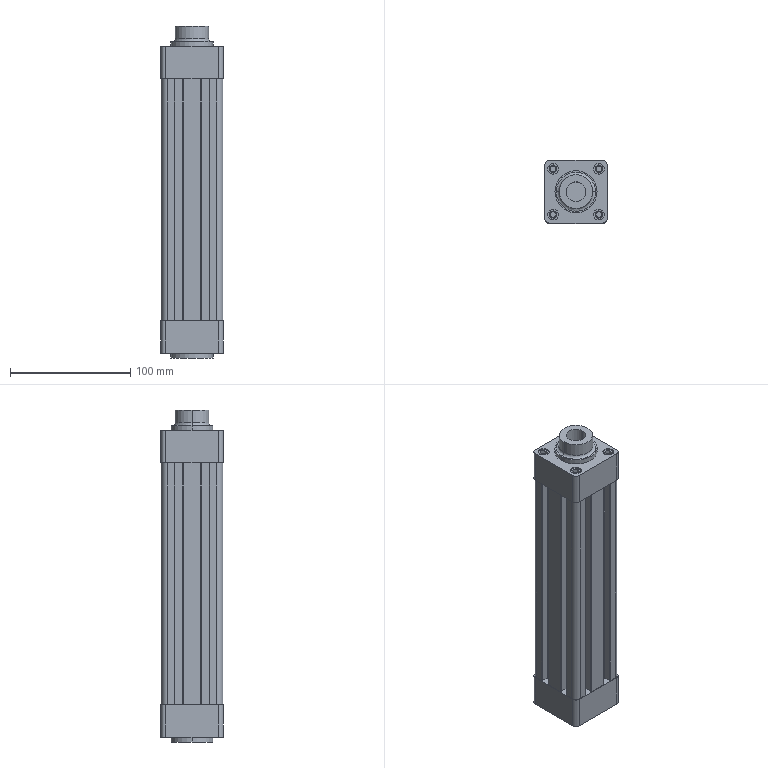Part | STEP file | fA_CP95SB40-150 (0) | 1 solid | 291 faces | box 52 x 52 x 276 mm | volume 568979 mm3 | plane 205 | cylinder 60 | cone 24 | torus 2 | commonest cylinder face diameters 4.773 x16 9 x16 8 x8 7.8 x4 10 x4 11.445 x4